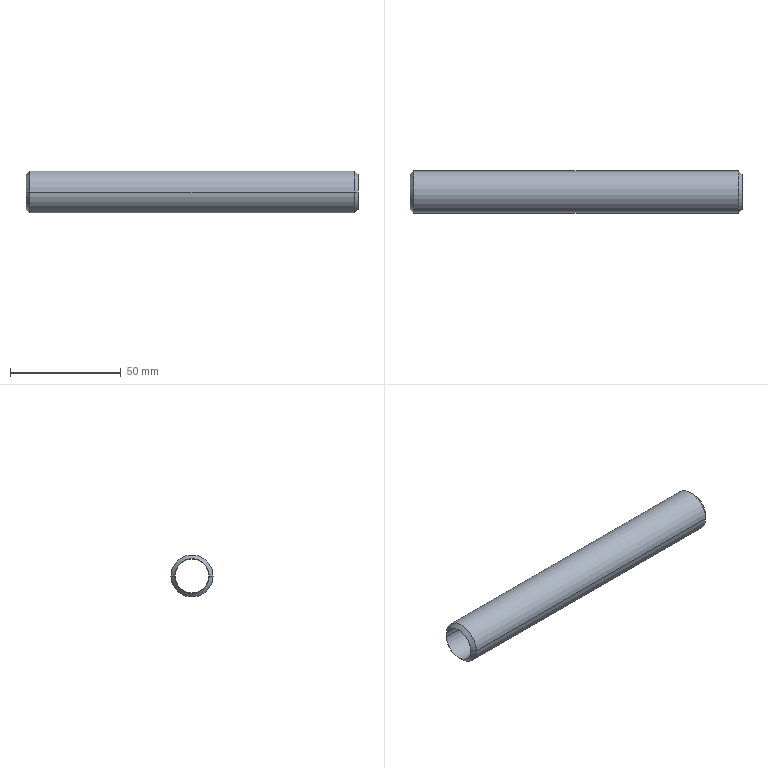Part | NX | features BREP 1 | 1 solid | 10 faces | box 149.86 x 19.05 x 19.05 mm | volume 15017 mm3 | cone 4 | cylinder 4 | plane 2 | commonest cylinder face diameters 15.291 x2 19.05 x2
STEP:
#1=CARTESIAN_POINT('',(-74.93,7.747,0.));
#2=VERTEX_POINT('',#1);
#3=CARTESIAN_POINT('',(-74.93,-7.747,0.));
#4=VERTEX_POINT('',#3);
#5=CARTESIAN_POINT('',(-74.93,0.,0.));
#6=DIRECTION('',(1.,0.,0.));
#7=DIRECTION('',(0.,1.,0.));
#8=AXIS2_PLACEMENT_3D('',#5,#6,#7);
#9=CIRCLE('',#8,7.747);
#10=EDGE_CURVE('',#2,#4,#9,.T.);
#11=ORIENTED_EDGE('',*,*,#10,.F.);
#12=CARTESIAN_POINT('',(-74.93,0.,0.));
#13=DIRECTION('',(1.,0.,0.));
#14=DIRECTION('',(0.,-1.,0.));
#15=AXIS2_PLACEMENT_3D('',#12,#13,#14);
#16=CIRCLE('',#15,7.747);
#17=EDGE_CURVE('',#4,#2,#16,.T.);
#18=ORIENTED_EDGE('',*,*,#17,.F.);
#19=EDGE_LOOP('',(#11,#18));
#20=FACE_BOUND('',#19,.T.);
#21=CARTESIAN_POINT('',(-74.93,7.645,0.));
#22=VERTEX_POINT('',#21);
#23=CARTESIAN_POINT('',(-74.93,-7.645,0.));
#24=VERTEX_POINT('',#23);
#25=CARTESIAN_POINT('',(-74.93,0.,0.));
#26=DIRECTION('',(-1.,0.,0.));
#27=DIRECTION('',(0.,1.,0.));
#28=AXIS2_PLACEMENT_3D('',#25,#26,#27);
#29=CIRCLE('',#28,7.645);
#30=EDGE_CURVE('',#22,#24,#29,.T.);
#31=ORIENTED_EDGE('',*,*,#30,.F.);
#32=CARTESIAN_POINT('',(-74.93,0.,0.));
#33=DIRECTION('',(-1.,0.,0.));
#34=DIRECTION('',(0.,-1.,0.));
#35=AXIS2_PLACEMENT_3D('',#32,#33,#34);
#36=CIRCLE('',#35,7.645);
#37=EDGE_CURVE('',#24,#22,#36,.T.);
#38=ORIENTED_EDGE('',*,*,#37,.F.);
#39=EDGE_LOOP('',(#31,#38));
#40=FACE_BOUND('',#39,.T.);
#41=CARTESIAN_POINT('',(-74.93,0.,0.));
#42=DIRECTION('',(1.,0.,0.));
#43=DIRECTION('',(0.,1.,0.));
#44=AXIS2_PLACEMENT_3D('',#41,#42,#43);
#45=PLANE('',#44);
#46=ADVANCED_FACE('',(#20,#40),#45,.F.);
#47=CARTESIAN_POINT('',(-73.152,9.525,0.));
#48=VERTEX_POINT('',#47);
#49=CARTESIAN_POINT('',(-74.93,7.747,0.));
#50=DIRECTION('',(0.7071,0.7071,0.));
#51=VECTOR('',#50,1000.);
#52=LINE('',#49,#51);
#53=EDGE_CURVE('',#48,#2,#52,.F.);
#54=ORIENTED_EDGE('',*,*,#53,.F.);
#55=CARTESIAN_POINT('',(-73.152,-9.525,0.));
#56=VERTEX_POINT('',#55);
#57=CARTESIAN_POINT('',(-73.152,0.,0.));
#58=DIRECTION('',(1.,0.,0.));
#59=DIRECTION('',(0.,-1.,0.));
#60=AXIS2_PLACEMENT_3D('',#57,#58,#59);
#61=CIRCLE('',#60,9.525);
#62=EDGE_CURVE('',#56,#48,#61,.T.);
#63=ORIENTED_EDGE('',*,*,#62,.F.);
#64=CARTESIAN_POINT('',(-74.93,-7.747,0.));
#65=DIRECTION('',(0.7071,-0.7071,0.));
#66=VECTOR('',#65,1000.);
#67=LINE('',#64,#66);
#68=EDGE_CURVE('',#56,#4,#67,.F.);
#69=ORIENTED_EDGE('',*,*,#68,.T.);
#70=ORIENTED_EDGE('',*,*,#17,.T.);
#71=EDGE_LOOP('',(#54,#63,#69,#70));
#72=FACE_BOUND('',#71,.T.);
#73=CARTESIAN_POINT('',(-74.041,0.,0.));
#74=DIRECTION('',(1.,0.,0.));
#75=DIRECTION('',(0.,-1.,0.));
#76=AXIS2_PLACEMENT_3D('',#73,#74,#75);
#77=CONICAL_SURFACE('',#76,8.636,0.7854);
#78=ADVANCED_FACE('',(#72),#77,.T.);
#79=ORIENTED_EDGE('',*,*,#68,.F.);
#80=CARTESIAN_POINT('',(-73.152,0.,0.));
#81=DIRECTION('',(1.,0.,0.));
#82=DIRECTION('',(0.,1.,0.));
#83=AXIS2_PLACEMENT_3D('',#80,#81,#82);
#84=CIRCLE('',#83,9.525);
#85=EDGE_CURVE('',#48,#56,#84,.T.);
#86=ORIENTED_EDGE('',*,*,#85,.F.);
#87=ORIENTED_EDGE('',*,*,#53,.T.);
#88=ORIENTED_EDGE('',*,*,#10,.T.);
#89=EDGE_LOOP('',(#79,#86,#87,#88));
#90=FACE_BOUND('',#89,.T.);
#91=CARTESIAN_POINT('',(-74.041,0.,0.));
#92=DIRECTION('',(1.,0.,0.));
#93=DIRECTION('',(0.,-1.,0.));
#94=AXIS2_PLACEMENT_3D('',#91,#92,#93);
#95=CONICAL_SURFACE('',#94,8.636,0.7854);
#96=ADVANCED_FACE('',(#90),#95,.T.);
#97=CARTESIAN_POINT('',(73.152,-9.525,0.));
#98=VERTEX_POINT('',#97);
#99=CARTESIAN_POINT('',(-73.152,-9.525,0.));
#100=DIRECTION('',(1.,0.,0.));
#101=VECTOR('',#100,1000.);
#102=LINE('',#99,#101);
#103=EDGE_CURVE('',#56,#98,#102,.T.);
#104=ORIENTED_EDGE('',*,*,#103,.T.);
#105=CARTESIAN_POINT('',(73.152,9.525,0.));
#106=VERTEX_POINT('',#105);
#107=CARTESIAN_POINT('',(73.152,0.,0.));
#108=DIRECTION('',(1.,0.,0.));
#109=DIRECTION('',(0.,1.,0.));
#110=AXIS2_PLACEMENT_3D('',#107,#108,#109);
#111=CIRCLE('',#110,9.525);
#112=EDGE_CURVE('',#106,#98,#111,.T.);
#113=ORIENTED_EDGE('',*,*,#112,.F.);
#114=CARTESIAN_POINT('',(-73.152,9.525,0.));
#115=DIRECTION('',(1.,0.,0.));
#116=VECTOR('',#115,1000.);
#117=LINE('',#114,#116);
#118=EDGE_CURVE('',#48,#106,#117,.T.);
#119=ORIENTED_EDGE('',*,*,#118,.F.);
#120=ORIENTED_EDGE('',*,*,#85,.T.);
#121=EDGE_LOOP('',(#104,#113,#119,#120));
#122=FACE_BOUND('',#121,.T.);
#123=CARTESIAN_POINT('',(-74.93,0.,0.));
#124=DIRECTION('',(1.,0.,0.));
#125=DIRECTION('',(0.,-1.,0.));
#126=AXIS2_PLACEMENT_3D('',#123,#124,#125);
#127=CYLINDRICAL_SURFACE('',#126,9.525);
#128=ADVANCED_FACE('',(#122),#127,.T.);
#129=ORIENTED_EDGE('',*,*,#118,.T.);
#130=CARTESIAN_POINT('',(73.152,0.,0.));
#131=DIRECTION('',(1.,0.,0.));
#132=DIRECTION('',(0.,-1.,0.));
#133=AXIS2_PLACEMENT_3D('',#130,#131,#132);
#134=CIRCLE('',#133,9.525);
#135=EDGE_CURVE('',#98,#106,#134,.T.);
#136=ORIENTED_EDGE('',*,*,#135,.F.);
#137=ORIENTED_EDGE('',*,*,#103,.F.);
#138=ORIENTED_EDGE('',*,*,#62,.T.);
#139=EDGE_LOOP('',(#129,#136,#137,#138));
#140=FACE_BOUND('',#139,.T.);
#141=CARTESIAN_POINT('',(-74.93,0.,0.));
#142=DIRECTION('',(1.,0.,0.));
#143=DIRECTION('',(0.,-1.,0.));
#144=AXIS2_PLACEMENT_3D('',#141,#142,#143);
#145=CYLINDRICAL_SURFACE('',#144,9.525);
#146=ADVANCED_FACE('',(#140),#145,.T.);
#147=CARTESIAN_POINT('',(74.93,-7.747,0.));
#148=VERTEX_POINT('',#147);
#149=CARTESIAN_POINT('',(74.93,-7.747,0.));
#150=DIRECTION('',(-0.7071,-0.7071,0.));
#151=VECTOR('',#150,1000.);
#152=LINE('',#149,#151);
#153=EDGE_CURVE('',#148,#98,#152,.T.);
#154=ORIENTED_EDGE('',*,*,#153,.T.);
#155=ORIENTED_EDGE('',*,*,#135,.T.);
#156=CARTESIAN_POINT('',(74.93,7.747,0.));
#157=VERTEX_POINT('',#156);
#158=CARTESIAN_POINT('',(74.93,7.747,0.));
#159=DIRECTION('',(-0.7071,0.7071,0.));
#160=VECTOR('',#159,1000.);
#161=LINE('',#158,#160);
#162=EDGE_CURVE('',#157,#106,#161,.T.);
#163=ORIENTED_EDGE('',*,*,#162,.F.);
#164=CARTESIAN_POINT('',(74.93,0.,0.));
#165=DIRECTION('',(1.,0.,0.));
#166=DIRECTION('',(0.,-1.,0.));
#167=AXIS2_PLACEMENT_3D('',#164,#165,#166);
#168=CIRCLE('',#167,7.747);
#169=EDGE_CURVE('',#148,#157,#168,.T.);
#170=ORIENTED_EDGE('',*,*,#169,.F.);
#171=EDGE_LOOP('',(#154,#155,#163,#170));
#172=FACE_BOUND('',#171,.T.);
#173=CARTESIAN_POINT('',(74.041,0.,0.));
#174=DIRECTION('',(-1.,0.,0.));
#175=DIRECTION('',(0.,1.,0.));
#176=AXIS2_PLACEMENT_3D('',#173,#174,#175);
#177=CONICAL_SURFACE('',#176,8.636,0.7854);
#178=ADVANCED_FACE('',(#172),#177,.T.);
#179=CARTESIAN_POINT('',(74.93,0.,0.));
#180=DIRECTION('',(1.,0.,0.));
#181=DIRECTION('',(0.,1.,0.));
#182=AXIS2_PLACEMENT_3D('',#179,#180,#181);
#183=CIRCLE('',#182,7.747);
#184=EDGE_CURVE('',#157,#148,#183,.T.);
#185=ORIENTED_EDGE('',*,*,#184,.T.);
#186=ORIENTED_EDGE('',*,*,#169,.T.);
#187=EDGE_LOOP('',(#185,#186));
#188=FACE_BOUND('',#187,.T.);
#189=CARTESIAN_POINT('',(74.93,7.645,0.));
#190=VERTEX_POINT('',#189);
#191=CARTESIAN_POINT('',(74.93,-7.645,0.));
#192=VERTEX_POINT('',#191);
#193=CARTESIAN_POINT('',(74.93,0.,0.));
#194=DIRECTION('',(-1.,0.,0.));
#195=DIRECTION('',(0.,1.,0.));
#196=AXIS2_PLACEMENT_3D('',#193,#194,#195);
#197=CIRCLE('',#196,7.645);
#198=EDGE_CURVE('',#190,#192,#197,.T.);
#199=ORIENTED_EDGE('',*,*,#198,.T.);
#200=CARTESIAN_POINT('',(74.93,0.,0.));
#201=DIRECTION('',(-1.,0.,0.));
#202=DIRECTION('',(0.,-1.,0.));
#203=AXIS2_PLACEMENT_3D('',#200,#201,#202);
#204=CIRCLE('',#203,7.645);
#205=EDGE_CURVE('',#192,#190,#204,.T.);
#206=ORIENTED_EDGE('',*,*,#205,.T.);
#207=EDGE_LOOP('',(#199,#206));
#208=FACE_BOUND('',#207,.T.);
#209=CARTESIAN_POINT('',(74.93,0.,0.));
#210=DIRECTION('',(1.,0.,0.));
#211=DIRECTION('',(0.,1.,0.));
#212=AXIS2_PLACEMENT_3D('',#209,#210,#211);
#213=PLANE('',#212);
#214=ADVANCED_FACE('',(#188,#208),#213,.T.);
#215=ORIENTED_EDGE('',*,*,#162,.T.);
#216=ORIENTED_EDGE('',*,*,#112,.T.);
#217=ORIENTED_EDGE('',*,*,#153,.F.);
#218=ORIENTED_EDGE('',*,*,#184,.F.);
#219=EDGE_LOOP('',(#215,#216,#217,#218));
#220=FACE_BOUND('',#219,.T.);
#221=CARTESIAN_POINT('',(74.041,0.,0.));
#222=DIRECTION('',(-1.,0.,0.));
#223=DIRECTION('',(0.,1.,0.));
#224=AXIS2_PLACEMENT_3D('',#221,#222,#223);
#225=CONICAL_SURFACE('',#224,8.636,0.7854);
#226=ADVANCED_FACE('',(#220),#225,.T.);
#227=CARTESIAN_POINT('',(-74.93,7.645,0.));
#228=DIRECTION('',(1.,0.,0.));
#229=VECTOR('',#228,1000.);
#230=LINE('',#227,#229);
#231=EDGE_CURVE('',#190,#22,#230,.F.);
#232=ORIENTED_EDGE('',*,*,#231,.F.);
#233=ORIENTED_EDGE('',*,*,#205,.F.);
#234=CARTESIAN_POINT('',(-74.93,-7.645,0.));
#235=DIRECTION('',(1.,0.,0.));
#236=VECTOR('',#235,1000.);
#237=LINE('',#234,#236);
#238=EDGE_CURVE('',#192,#24,#237,.F.);
#239=ORIENTED_EDGE('',*,*,#238,.T.);
#240=ORIENTED_EDGE('',*,*,#37,.T.);
#241=EDGE_LOOP('',(#232,#233,#239,#240));
#242=FACE_BOUND('',#241,.T.);
#243=CARTESIAN_POINT('',(-74.93,0.,0.));
#244=DIRECTION('',(1.,0.,0.));
#245=DIRECTION('',(0.,-1.,0.));
#246=AXIS2_PLACEMENT_3D('',#243,#244,#245);
#247=CYLINDRICAL_SURFACE('',#246,7.645);
#248=ADVANCED_FACE('',(#242),#247,.F.);
#249=ORIENTED_EDGE('',*,*,#238,.F.);
#250=ORIENTED_EDGE('',*,*,#198,.F.);
#251=ORIENTED_EDGE('',*,*,#231,.T.);
#252=ORIENTED_EDGE('',*,*,#30,.T.);
#253=EDGE_LOOP('',(#249,#250,#251,#252));
#254=FACE_BOUND('',#253,.T.);
#255=CARTESIAN_POINT('',(-74.93,0.,0.));
#256=DIRECTION('',(1.,0.,0.));
#257=DIRECTION('',(0.,-1.,0.));
#258=AXIS2_PLACEMENT_3D('',#255,#256,#257);
#259=CYLINDRICAL_SURFACE('',#258,7.645);
#260=ADVANCED_FACE('',(#254),#259,.F.);
#261=CLOSED_SHELL('',(#46,#78,#96,#128,#146,#178,#214,#226,#248,#260));
#262=MANIFOLD_SOLID_BREP('',#261);
#263=(LENGTH_UNIT()NAMED_UNIT(*)SI_UNIT(.MILLI.,.METRE.));
#264=UNCERTAINTY_MEASURE_WITH_UNIT(LENGTH_MEASURE(0.00001),#263,'','');
#265=(NAMED_UNIT(*)PLANE_ANGLE_UNIT()SI_UNIT($,.RADIAN.));
#266=(NAMED_UNIT(*)SI_UNIT($,.STERADIAN.)SOLID_ANGLE_UNIT());
#267=(GEOMETRIC_REPRESENTATION_CONTEXT(3)GLOBAL_UNCERTAINTY_ASSIGNED_CONTEXT((#264))GLOBAL_UNIT_ASSIGNED_CONTEXT((#263,#265,#266))REPRESENTATION_CONTEXT('',''));
#268=ADVANCED_BREP_SHAPE_REPRESENTATION('',(#262),#267);